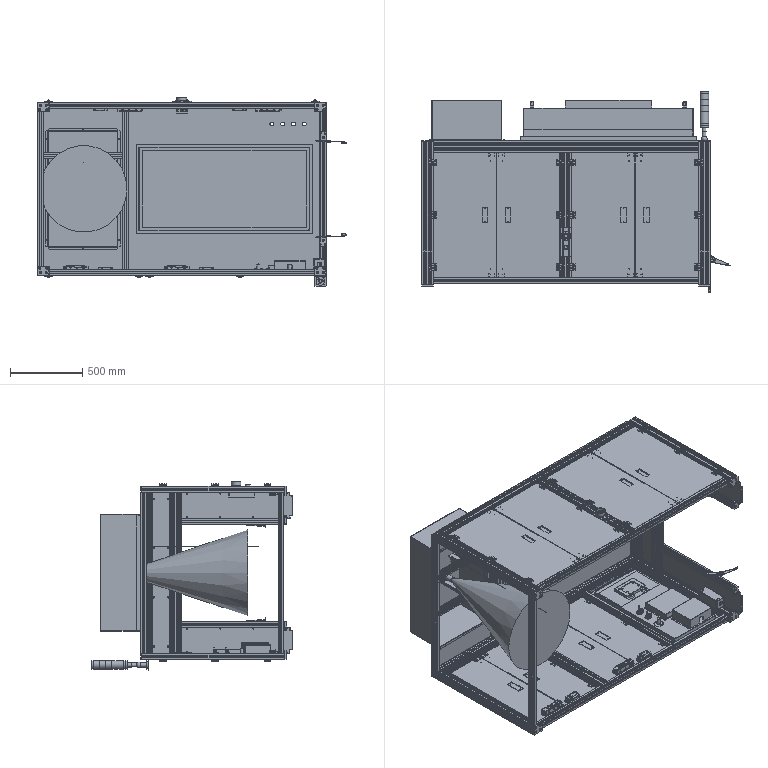Part | NX | 241 solids | 10395 faces | volume 307084215 mm3 | plane 7225 | cylinder 2416 | cone 368 | spline 343 | torus 26 | sphere 17 | commonest cylinder face diameters 4 x225 8 x219 6 x194 6.5 x133 2.5 x130 3.3 x118